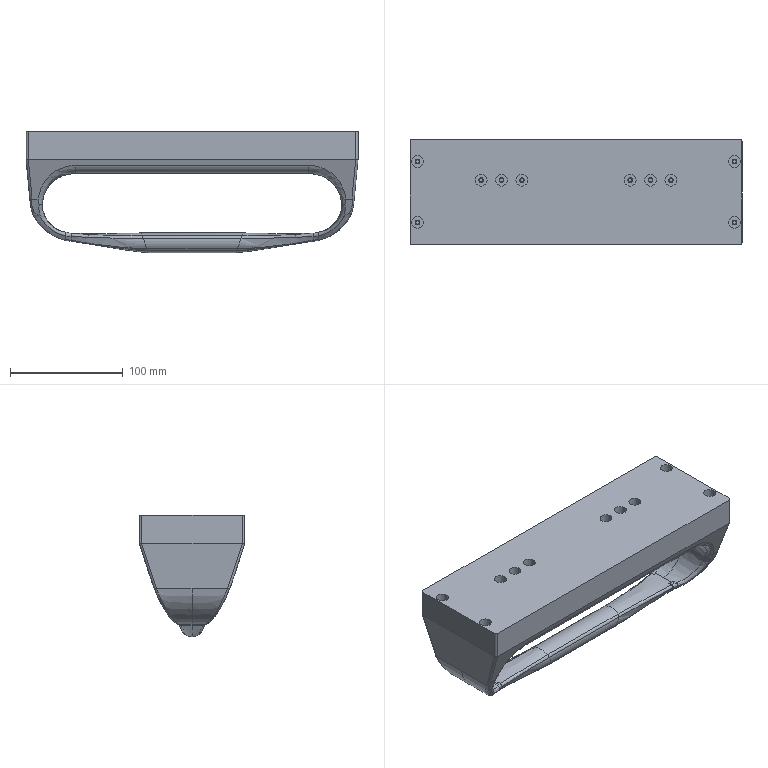CAM job | NX | 3+2 milling, drilling | part box 294.078 x 93.5 x 107.5 mm
Operations:
program,operation,operation_type,tool,method,geometry_group,spindle_rpm,surface_speed,feed_per_tooth,feed_cut,feed_plunge,cut_length_mm,path_length_mm,cut_time_min,machine_time_min
1,FLOOR_WALL,VolumeBased25DMillingOperation,D63,METHOD,A,6500.0,1286.0,0.0962,1250.0,100.0,1191.531,1242.531,0.9532,0.9583
1,ADAPTIVE_MILLING,CavityMilling,D10,METHOD,A,7500.0,235.0,0.2,3000.0,1000.0,55601.825,57291.872,19.075,19.244
1,DRILLING_COPY_1,Operation,D6A45,METHOD,A,5000.0,94.0,0.025,250.0,0.0,51.0,583.914,0.204,0.2573
1,DRILLING_COPY_COPY_1,Operation,3.2ZT,METHOD,A,2000.0,15.0,0.03,120.0,0.0,144.614,771.142,1.205,1.268
1,DRILLING_COPY_COPY_1_COPY,Operation,M4,METHOD,A,200.0,2.0,0.0017,0.7,0.0,130.0,741.914,185.714,185.775
1,FLOOR_WALL_1_1_COPY,VolumeBased25DMillingOperation,D10JING,METHOD,A,7500.0,235.0,0.0833,1250.0,100.0,7122.009,9301.685,5.698,5.916
1,ZLEVEL_PROFILE_COPY_COPY_1_COPY_COPY_COPY,ZLevelMilling,D10JING,METHOD,A,7500.0,235.0,0.0667,1000.0,100.0,812.205,906.205,0.8122,0.8216
1,ZLEVEL_PROFILE_COPY_COPY_1_COPY_COPY_COPY_COPY,ZLevelMilling,D10JING,METHOD,A,7500.0,235.0,0.0667,1000.0,100.0,38.707,116.707,0.0387,0.0465
1,ZLEVEL_PROFILE_COPY_1_COPY_1_COPY_1_1,ZLevelMilling,D6,METHOD,A,7500.0,141.0,0.2,3000.0,800.0,23656.823,24054.311,7.891,7.931
1,ZLEVEL_PROFILE_1_COPY_1_COPY_COPY_1,ZLevelMilling,D6A45,METHOD,A,7500.0,141.0,0.0667,1000.0,100.0,1779.142,2416.652,1.779,1.843
1,ZLEVEL_PROFILE_1_COPY_1_COPY_COPY_1_COPY,ZLevelMilling,D6A45,METHOD,A,7500.0,141.0,0.0667,1000.0,100.0,56.688,136.688,0.0567,0.0647
2,ADAPTIVE_MILLING_COPY,CavityMilling,D10,METHOD,B,7500.0,235.0,0.2,3000.0,1000.0,118050.561,211714.127,40.196,49.563
2,ZLEVEL_PROFILE_COPY_COPY_1_COPY_COPY_COPY_COPY_1_COPY,ZLevelMilling,D10JING,METHOD,MCS_MILL_B,7500.0,235.0,0.0667,1000.0,100.0,1305.003,2275.66,1.305,1.402
2,ZLEVEL_PROFILE_COPY_COPY_1_COPY_COPY_COPY_COPY_1,ZLevelMilling,D10JING,METHOD,B,7500.0,235.0,0.0667,1000.0,100.0,1703.981,2061.046,1.704,1.74
2,FIXED_CONTOUR,SurfaceContour,D10R2,METHOD,MCS_MILL_B,7500.0,188.0,0.1667,2500.0,1000.0,234717.23,236063.189,93.938,94.072
2,ZLEVEL_PROFILE_COPY_1_COPY_1_COPY_1_1_1,ZLevelMilling,D10R2,METHOD,B,7500.0,235.0,0.1333,2000.0,1000.0,19639.034,21130.053,9.836,9.986
2,ZLEVEL_PROFILE_COPY_1_COPY_1_COPY_1_1_1_COPY,ZLevelMilling,D10R2,METHOD,B,7500.0,235.0,0.1333,2000.0,1000.0,38364.479,39292.603,19.193,19.286
3,ADAPTIVE_MILLING_COPY_COPY,CavityMilling,D10,METHOD,C,7500.0,235.0,0.2,3000.0,1000.0,118720.482,211559.009,40.416,49.7
3,ZLEVEL_PROFILE_COPY_COPY_1_COPY_COPY_COPY_COPY_1_COPY_COPY,ZLevelMilling,D10JING,METHOD,MCS_MILL_C,7500.0,235.0,0.0667,1000.0,100.0,1304.982,2272.139,1.305,1.402
3,ZLEVEL_PROFILE_COPY_COPY_1_COPY_COPY_COPY_COPY_1_COPY_1,ZLevelMilling,D10JING,METHOD,C,7500.0,235.0,0.0667,1000.0,100.0,1704.739,2062.394,1.705,1.74
3,FIXED_CONTOUR_COPY_1,SurfaceContour,D10R2,METHOD,MCS_MILL_C,7500.0,188.0,0.1667,2500.0,1000.0,233426.829,235258.726,93.412,93.596
3,ZLEVEL_PROFILE_COPY_1_COPY_1_COPY_1_1_1_COPY_1,ZLevelMilling,D10R2,METHOD,C,7500.0,235.0,0.1333,2000.0,1000.0,19764.683,21296.315,9.899,10.053
3,ZLEVEL_PROFILE_COPY_1_COPY_1_COPY_1_1_1_COPY_COPY,ZLevelMilling,D10R2,METHOD,C,7500.0,235.0,0.1333,2000.0,1000.0,38368.692,39663.814,19.197,19.327
4夹具1夹-301-95-30,FLOOR_WALL_COPY,VolumeBased25DMillingOperation,D63,METHOD,D,6500.0,1286.0,0.0962,1250.0,100.0,1181.531,1235.531,0.9452,0.9506
4夹具1夹-301-95-30,DRILLING_COPY_1_COPY,Operation,D6A45,METHOD,D,5000.0,94.0,0.025,250.0,0.0,51.0,583.876,0.204,0.2573
4夹具1夹-301-95-30,DRILLING_COPY_COPY_1_COPY_1,Operation,4.3ZT,METHOD,D,2000.0,15.0,0.03,120.0,0.0,295.618,1073.112,2.463,2.541
4夹具1夹-301-95-30,HOLE_MILLING,CylinderMilling,D6,METHOD,D,7000.0,131.0,0.0929,1300.0,100.0,5692.402,6839.879,4.379,4.494
4夹具1夹-301-95-30,ADAPTIVE_MILLING_COPY_COPY_COPY,CavityMilling,D10,METHOD,D,7500.0,235.0,0.2,3000.0,1000.0,7280.775,7477.516,2.428,2.448
4夹具1夹-301-95-30,ZLEVEL_PROFILE_COPY_COPY_1_COPY_COPY_COPY_COPY_1_COPY_COPY_COPY,ZLevelMilling,D10JING,METHOD,D,7500.0,235.0,0.0667,1000.0,100.0,1624.406,1809.666,1.624,1.643
4夹具1夹-301-95-30,ZLEVEL_PROFILE_1_COPY_1_COPY_COPY_1_COPY_1,ZLevelMilling,D6A45,METHOD,D,7500.0,141.0,0.0667,1000.0,100.0,1111.185,3453.175,1.111,1.345
5夹具2夹-301-95-30,FLOOR_WALL_COPY_COPY,VolumeBased25DMillingOperation,D63,METHOD,E,6500.0,1286.0,0.0962,1250.0,100.0,1181.531,1235.531,0.9452,0.9506
5夹具2夹-301-95-30,ADAPTIVE_MILLING_COPY_COPY_COPY_COPY,CavityMilling,D10,METHOD,E,7500.0,235.0,0.2,3000.0,1000.0,13617.516,18658.106,4.55,5.054
5夹具2夹-301-95-30,ADAPTIVE_MILLING_COPY_COPY_COPY_COPY_COPY,CavityMilling,D10,METHOD,E,7500.0,235.0,0.2,3000.0,1000.0,4307.759,4591.991,2.036,2.064
5夹具2夹-301-95-30,ZLEVEL_PROFILE_COPY_1_COPY_1_COPY_1_1_COPY_COPY_COPY_1,ZLevelMilling,D6,METHOD,E,7500.0,141.0,0.1,1500.0,800.0,1453.828,3458.513,1.159,1.359
5夹具2夹-301-95-30,FLOOR_WALL_1_1_COPY_COPY,VolumeBased25DMillingOperation,D6,METHOD,E,7500.0,235.0,0.0833,1250.0,100.0,4077.337,4798.826,3.262,3.334
5夹具2夹-301-95-30,ZLEVEL_PROFILE_1_COPY_1_COPY_COPY_1_COPY_1_COPY,ZLevelMilling,D6A45,METHOD,E,7500.0,141.0,0.0667,1000.0,100.0,962.34,1495.464,0.9623,1.016
5夹具2夹-301-95-30,ZLEVEL_PROFILE_1_COPY_1_COPY_COPY_1_COPY_1_COPY_COPY,ZLevelMilling,D6A45,METHOD,E,7500.0,141.0,0.0667,1000.0,100.0,814.413,1853.745,0.8144,0.9183
5夹具2夹-301-95-30,刀补5,VolumeBased25DMillingOperation,D6,METHOD,E,7500.0,235.0,0.0667,1000.0,100.0,955.436,1306.752,0.9554,0.9906